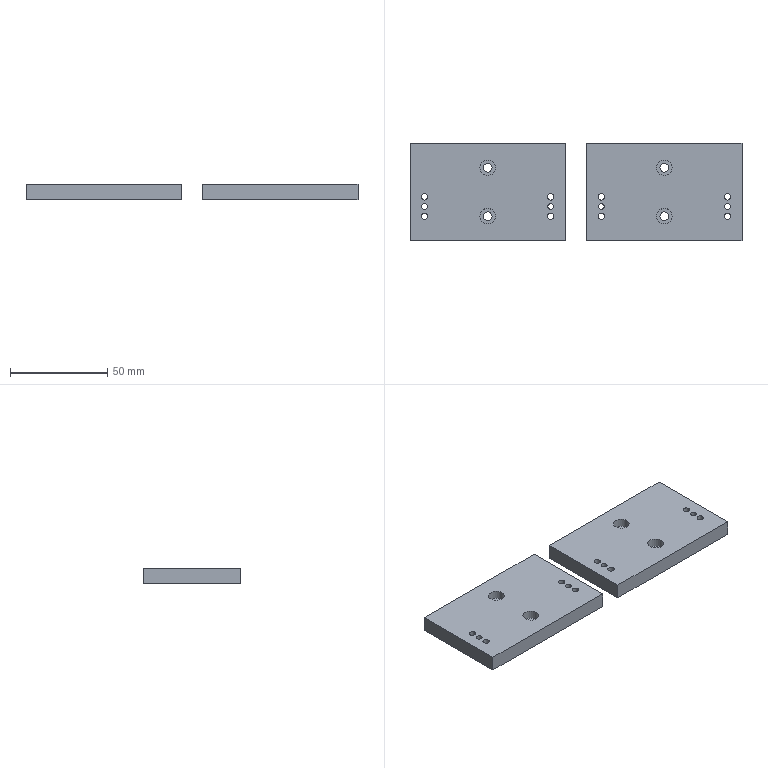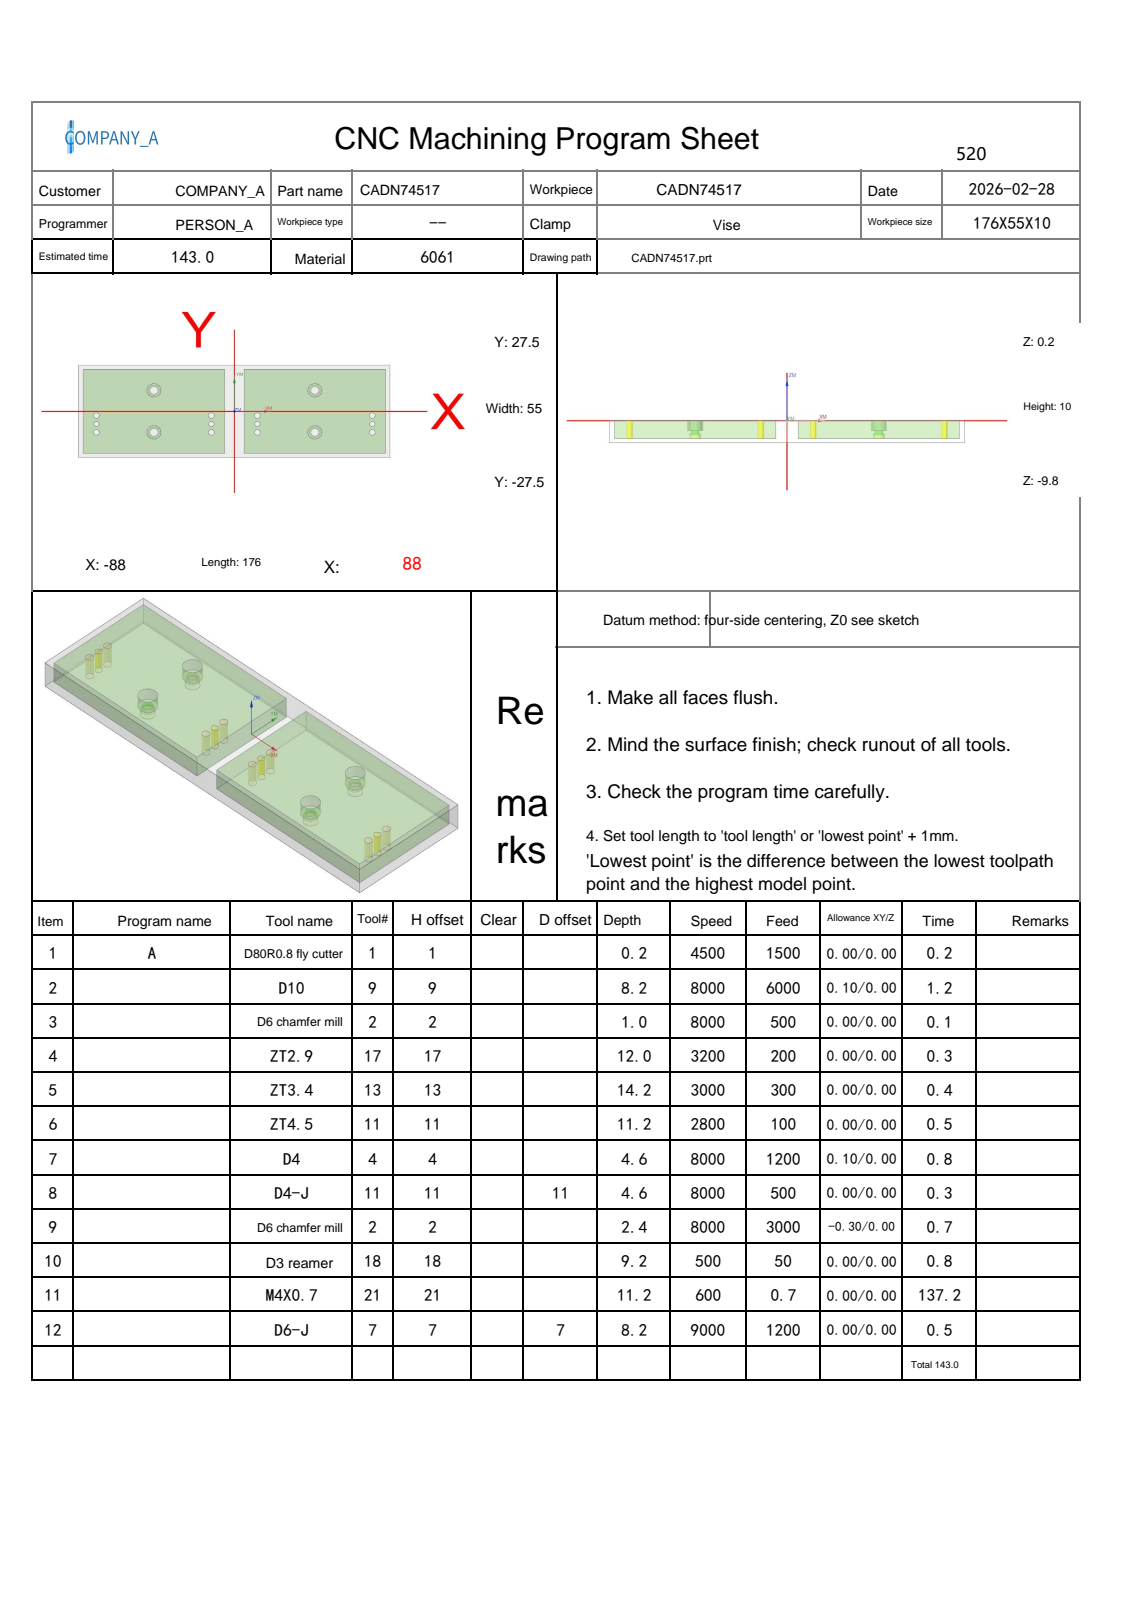NC program | NX | posted by the shop | part box 171 x 50 x 8 mm
Whole program:
%
O0001
(Machine time: 271.00 MIN)
(===Total Tool:10===)
(T1=D80R0.8 fly cutter D=80.  R=0.8  D-  H01 Z=0.    )
(T9=D10     D=10.  R=0.   D-  H09 Z=-8.   )
(T2=D6 chamfer mill   D=6.   R=0.   D-  H02 Z=-2.2  )
(T17=ZT2.9  D=2.9  DR_a=120 D-  H17 Z=-11.84)
(T13=ZT3.4  D=3.4  DR_a=118 D-  H13 Z=-14.  )
(T11=ZT4.5  D=4.5  DR_a=118 D-  H11 Z=-11.  )
(T4=D4      D=4.   R=0.   D-  H04 Z=-4.4  )
(T18=D3 reamer   D=3.   DR_a=180 D-  H18 Z=-9.   )
(T21=M4X0.7 D=3.3  DR_a=180 D-  H21 Z=-11.  )
(T7=D6-J    D=6.   R=0.   D7  H07 Z=-8.   )
G80 G90 G17 G49 G40
G91 G28 Z0
M01
N1 T01 M06
(D80R0.8 fly cutter  D=80. R=0.8 H=01 ce=0.00 di=0.00)
G00 G90 G54 X-130.5 Y0.0 M03 S4500
G43 H01 Z50.
M08
Z2.
G01 Z0.0 F1500.
X-125.5
X125.5
X130.5
Z2.
G00 Z50.
G91 G28 Z0.0
M05
M09
G91 G28 Z0.0
M01
N2 T09 M06
(D10  D=10. R=0. H=09 ce=0.10 di=0.00)
G00 G90 G54 X-45.5 Y-30.1 M03 S8000
G43 H09 Z50.
M08
Z.5
G01 X-85.5 Z.394 F6000.
G02 X-90.6 Y-25. Z.373 I0.0 J5.1
G01 Y25. Z.241
G02 X-85.5 Y30.1 Z.219 I5.1 J0.0
G01 X-5.5 Z.008
G02 X-.4 Y25. Z-.013 I0.0 J-5.1
G01 Y-25. Z-.146
G02 X-5.5 Y-30.1 Z-.167 I-5.1 J0.0
G01 X-85.5 Z-.379
G02 X-90.6 Y-25. Z-.4 I0.0 J5.1
G01 Y25. Z-.532
G02 X-85.5 Y30.1 Z-.553 I5.1 J0.0
G01 X-5.5 Z-.765
G02 X-.4 Y25. Z-.786 I0.0 J-5.1
G01 Y-25. Z-.918
G02 X-5.5 Y-30.1 Z-.94 I-5.1 J0.0
G01 X-85.5 Z-1.151
G02 X-90.6 Y-25. Z-1.172 I0.0 J5.1
G01 Y25. Z-1.305
G02 X-85.5 Y30.1 Z-1.326 I5.1 J0.0
G01 X-5.5 Z-1.538
G02 X-.4 Y25. Z-1.559 I0.0 J-5.1
G01 Y-25. Z-1.691
G02 X-5.5 Y-30.1 Z-1.712 I-5.1 J0.0
G01 X-85.5 Z-1.924
G02 X-90.6 Y-25. Z-1.945 I0.0 J5.1
G01 Y25. Z-2.078
G02 X-85.5 Y30.1 Z-2.099 I5.1 J0.0
G01 X-5.5 Z-2.31
G02 X-.4 Y25. Z-2.332 I0.0 J-5.1
G01 Y-25. Z-2.464
G02 X-5.5 Y-30.1 Z-2.485 I-5.1 J0.0
G01 X-85.5 Z-2.697
G02 X-90.6 Y-25. Z-2.718 I0.0 J5.1
G01 Y25. Z-2.85
G02 X-85.5 Y30.1 Z-2.871 I5.1 J0.0
G01 X-5.5 Z-3.083
G02 X-.4 Y25. Z-3.104 I0.0 J-5.1
G01 Y-25. Z-3.237
G02 X-5.5 Y-30.1 Z-3.258 I-5.1 J0.0
G01 X-85.5 Z-3.469
G02 X-90.6 Y-25. Z-3.491 I0.0 J5.1
G01 Y25. Z-3.623
G02 X-85.5 Y30.1 Z-3.644 I5.1 J0.0
G01 X-5.5 Z-3.856
G02 X-.4 Y25. Z-3.877 I0.0 J-5.1
G01 Y-25. Z-4.009
G02 X-5.5 Y-30.1 Z-4.031 I-5.1 J0.0
G01 X-85.5 Z-4.242
G02 X-90.6 Y-25. Z-4.263 I0.0 J5.1
G01 Y25. Z-4.396
G02 X-85.5 Y30.1 Z-4.417 I5.1 J0.0
G01 X-5.5 Z-4.629
G02 X-.4 Y25. Z-4.65 I0.0 J-5.1
G01 Y-25. Z-4.782
G02 X-5.5 Y-30.1 Z-4.803 I-5.1 J0.0
G01 X-85.5 Z-5.015
G02 X-90.6 Y-25. Z-5.036 I0.0 J5.1
G01 Y25. Z-5.168
G02 X-85.5 Y30.1 Z-5.19 I5.1 J0.0
G01 X-5.5 Z-5.401
G02 X-.4 Y25. Z-5.422 I0.0 J-5.1
G01 Y-25. Z-5.555
G02 X-5.5 Y-30.1 Z-5.576 I-5.1 J0.0
G01 X-85.5 Z-5.788
G02 X-90.6 Y-25. Z-5.809 I0.0 J5.1
G01 Y25. Z-5.941
G02 X-85.5 Y30.1 Z-5.962 I5.1 J0.0
G01 X-5.5 Z-6.174
G02 X-.4 Y25. Z-6.195 I0.0 J-5.1
G01 Y-25. Z-6.328
G02 X-5.5 Y-30.1 Z-6.349 I-5.1 J0.0
G01 X-85.5 Z-6.56
G02 X-90.6 Y-25. Z-6.582 I0.0 J5.1
G01 Y25. Z-6.714
G02 X-85.5 Y30.1 Z-6.735 I5.1 J0.0
G01 X-5.5 Z-6.947
G02 X-.4 Y25. Z-6.968 I0.0 J-5.1
G01 Y-25. Z-7.1
G02 X-5.5 Y-30.1 Z-7.121 I-5.1 J0.0
G01 X-85.5 Z-7.333
G02 X-90.6 Y-25. Z-7.354 I0.0 J5.1
G01 Y25. Z-7.487
G02 X-85.5 Y30.1 Z-7.508 I5.1 J0.0
G01 X-5.5 Z-7.719
G02 X-.4 Y25. Z-7.741 I0.0 J-5.1
G01 Y-25. Z-7.873
G02 X-5.5 Y-30.1 Z-7.894 I-5.1 J0.0
G01 X-45.5 Z-8.
X-85.5
G02 X-90.6 Y-25. I0.0 J5.1
G01 Y25.
G02 X-85.5 Y30.1 I5.1 J0.0
G01 X-5.5
G02 X-.4 Y25. I0.0 J-5.1
G01 Y-25.
G02 X-5.5 Y-30.1 I-5.1 J0.0
G01 X-45.5
X-46.
Z-7.
G00 Z50.
X45.5
Z.5
G01 X5.5 Z.394
G02 X.4 Y-25. Z.373 I0.0 J5.1
G01 Y25. Z.241
G02 X5.5 Y30.1 Z.219 I5.1 J0.0
G01 X85.5 Z.008
G02 X90.6 Y25. Z-.013 I0.0 J-5.1
G01 Y-25. Z-.146
G02 X85.5 Y-30.1 Z-.167 I-5.1 J0.0
G01 X5.5 Z-.379
G02 X.4 Y-25. Z-.4 I0.0 J5.1
G01 Y25. Z-.532
G02 X5.5 Y30.1 Z-.553 I5.1 J0.0
G01 X85.5 Z-.765
G02 X90.6 Y25. Z-.786 I0.0 J-5.1
G01 Y-25. Z-.918
G02 X85.5 Y-30.1 Z-.94 I-5.1 J0.0
G01 X5.5 Z-1.151
G02 X.4 Y-25. Z-1.172 I0.0 J5.1
G01 Y25. Z-1.305
G02 X5.5 Y30.1 Z-1.326 I5.1 J0.0
G01 X85.5 Z-1.538
G02 X90.6 Y25. Z-1.559 I0.0 J-5.1
G01 Y-25. Z-1.691
G02 X85.5 Y-30.1 Z-1.712 I-5.1 J0.0
G01 X5.5 Z-1.924
G02 X.4 Y-25. Z-1.945 I0.0 J5.1
G01 Y25. Z-2.078
G02 X5.5 Y30.1 Z-2.099 I5.1 J0.0
G01 X85.5 Z-2.31
G02 X90.6 Y25. Z-2.332 I0.0 J-5.1
G01 Y-25. Z-2.464
G02 X85.5 Y-30.1 Z-2.485 I-5.1 J0.0
G01 X5.5 Z-2.697
G02 X.4 Y-25. Z-2.718 I0.0 J5.1
G01 Y25. Z-2.85
G02 X5.5 Y30.1 Z-2.871 I5.1 J0.0
G01 X85.5 Z-3.083
G02 X90.6 Y25. Z-3.104 I0.0 J-5.1
G01 Y-25. Z-3.237
G02 X85.5 Y-30.1 Z-3.258 I-5.1 J0.0
G01 X5.5 Z-3.469
G02 X.4 Y-25. Z-3.491 I0.0 J5.1
G01 Y25. Z-3.623
G02 X5.5 Y30.1 Z-3.644 I5.1 J0.0
G01 X85.5 Z-3.856
G02 X90.6 Y25. Z-3.877 I0.0 J-5.1
G01 Y-25. Z-4.009
G02 X85.5 Y-30.1 Z-4.031 I-5.1 J0.0
G01 X5.5 Z-4.242
G02 X.4 Y-25. Z-4.263 I0.0 J5.1
G01 Y25. Z-4.396
G02 X5.5 Y30.1 Z-4.417 I5.1 J0.0
G01 X85.5 Z-4.629
G02 X90.6 Y25. Z-4.65 I0.0 J-5.1
G01 Y-25. Z-4.782
G02 X85.5 Y-30.1 Z-4.803 I-5.1 J0.0
G01 X5.5 Z-5.015
G02 X.4 Y-25. Z-5.036 I0.0 J5.1
G01 Y25. Z-5.168
G02 X5.5 Y30.1 Z-5.19 I5.1 J0.0
G01 X85.5 Z-5.401
G02 X90.6 Y25. Z-5.422 I0.0 J-5.1
G01 Y-25. Z-5.555
G02 X85.5 Y-30.1 Z-5.576 I-5.1 J0.0
G01 X5.5 Z-5.788
G02 X.4 Y-25. Z-5.809 I0.0 J5.1
G01 Y25. Z-5.941
G02 X5.5 Y30.1 Z-5.962 I5.1 J0.0
G01 X85.5 Z-6.174
G02 X90.6 Y25. Z-6.195 I0.0 J-5.1
G01 Y-25. Z-6.328
G02 X85.5 Y-30.1 Z-6.349 I-5.1 J0.0
G01 X5.5 Z-6.56
G02 X.4 Y-25. Z-6.582 I0.0 J5.1
G01 Y25. Z-6.714
G02 X5.5 Y30.1 Z-6.735 I5.1 J0.0
G01 X85.5 Z-6.947
G02 X90.6 Y25. Z-6.968 I0.0 J-5.1
G01 Y-25. Z-7.1
G02 X85.5 Y-30.1 Z-7.121 I-5.1 J0.0
G01 X5.5 Z-7.333
G02 X.4 Y-25. Z-7.354 I0.0 J5.1
G01 Y25. Z-7.487
G02 X5.5 Y30.1 Z-7.508 I5.1 J0.0
G01 X85.5 Z-7.719
G02 X90.6 Y25. Z-7.741 I0.0 J-5.1
G01 Y-25. Z-7.873
G02 X85.5 Y-30.1 Z-7.894 I-5.1 J0.0
G01 X45.5 Z-8.
X5.5
G02 X.4 Y-25. I0.0 J5.1
G01 Y25.
G02 X5.5 Y30.1 I5.1 J0.0
G01 X85.5
G02 X90.6 Y25. I0.0 J-5.1
G01 Y-25.
G02 X85.5 Y-30.1 I-5.1 J0.0
G01 X45.5
X45.
Z-7.
G00 Z50.
G91 G28 Z0.0
M05
M09
G91 G28 Z0.0
M01
N3 T02 M06
(D6 chamfer mill  D=6. R=0. H=02 ce=0.00 di=0.00)
G00 G90 G54 X-78. Y-2.5 M03 S8000
G43 H02 Z50.
M08
G98 G81 X-78. Y-2.5 Z-.8 R1. F500.
Y-7.5
Y-12.5
X-45.5
Y12.5
X-13. Y-2.5
Y-7.5
Y-12.5
X13.
Y-7.5
Y-2.5
X45.5 Y12.5
Y-12.5
X78.
Y-7.5
Y-2.5
G80
G00 Z50.
G91 G28 Z0.0
M05
M09
G91 G28 Z0.0
M01
N4 T17 M06
(ZT2.9 D=2.9 DR_a=120 H=17)
G00 G90 G54 X78. Y-7.5 M03 S3200
G43 H17 Z50.
M08
G98 G83 X78. Y-7.5 Z-11.837 R1. F200. Q2.
X13.
X-13.
X-78.
G80
G00 Z50.
G91 G28 Z0.0
M05
M09
G91 G28 Z0.0
M01
N5 T13 M06
(ZT3.4 D=3.4 DR_a=118 H=13)
G00 G90 G54 X-78. Y-12.5 M03 S3000
G43 H13 Z50.
M08
G98 G83 X-78. Y-12.5 Z-14. R1. F300. Q2.
Y-2.5
X-13.
Y-12.5
X13.
Y-2.5
X78.
Y-12.5
G80
G00 Z50.
G91 G28 Z0.0
M05
M09
G91 G28 Z0.0
M01
N6 T11 M06
(ZT4.5 D=4.5 DR_a=118 H=11)
G00 G90 G54 X45.5 Y-12.5 M03 S2800
G43 H11 Z50.
M08
G98 G83 X45.5 Y-12.5 Z-11. R1. F100. Q2.
Y12.5
X-45.5
Y-12.5
G80
G00 Z50.
G91 G28 Z0.0
M05
M09
G91 G28 Z0.0
M01
N7 T04 M06
(D4  D=4. R=0. H=04 ce=0.10 di=0.00)
G00 G90 G54 X45.5 Y-12.5 M03 S8000
G43 H04 Z50.
M08
Z.5
G03 X46.45 Y-13.45 I.95 J0.0 F1200.
X47.4 Y-12.5 I0.0 J.95
X47.4 Y-12.5 Z.2 I-1.9 J0.0
X47.4 Y-12.5 Z-.1 I-1.9 J0.0
X47.4 Y-12.5 Z-.4 I-1.9 J0.0
X47.4 Y-12.5 Z-.7 I-1.9 J0.0
X47.4 Y-12.5 Z-1. I-1.9 J0.0
X47.4 Y-12.5 Z-1.3 I-1.9 J0.0
X47.4 Y-12.5 Z-1.6 I-1.9 J0.0
X47.4 Y-12.5 Z-1.9 I-1.9 J0.0
X47.4 Y-12.5 Z-2.2 I-1.9 J0.0
X47.4 Y-12.5 Z-2.5 I-1.9 J0.0
X47.4 Y-12.5 Z-2.8 I-1.9 J0.0
X47.4 Y-12.5 Z-3.1 I-1.9 J0.0
X47.4 Y-12.5 Z-3.4 I-1.9 J0.0
X47.4 Y-12.5 Z-3.7 I-1.9 J0.0
X47.4 Y-12.5 Z-4. I-1.9 J0.0
X47.4 Y-12.5 Z-4.3 I-1.9 J0.0
X44.55 Y-10.855 Z-4.4 I-1.9 J0.0
X43.6 Y-12.5 I.95 J-1.645
X45.5 Y-14.4 I1.9 J0.0
X47.4 Y-12.5 I0.0 J1.9
X45.5 Y-10.6 I-1.9 J0.0
X44.55 Y-10.855 I0.0 J-1.9
X44.075 Y-11.677 I.475 J-.823
X45.025 Y-12.627 I.95 J0.0
X45.5 Y-12.5 I0.0 J.95
G00 Z50.
Y12.5
Z.5
G03 X46.45 Y11.55 I.95 J0.0
X47.4 Y12.5 I0.0 J.95
X47.4 Y12.5 Z.2 I-1.9 J0.0
X47.4 Y12.5 Z-.1 I-1.9 J0.0
X47.4 Y12.5 Z-.4 I-1.9 J0.0
X47.4 Y12.5 Z-.7 I-1.9 J0.0
X47.4 Y12.5 Z-1. I-1.9 J0.0
X47.4 Y12.5 Z-1.3 I-1.9 J0.0
X47.4 Y12.5 Z-1.6 I-1.9 J0.0
X47.4 Y12.5 Z-1.9 I-1.9 J0.0
X47.4 Y12.5 Z-2.2 I-1.9 J0.0
X47.4 Y12.5 Z-2.5 I-1.9 J0.0
X47.4 Y12.5 Z-2.8 I-1.9 J0.0
X47.4 Y12.5 Z-3.1 I-1.9 J0.0
X47.4 Y12.5 Z-3.4 I-1.9 J0.0
X47.4 Y12.5 Z-3.7 I-1.9 J0.0
X47.4 Y12.5 Z-4. I-1.9 J0.0
X47.4 Y12.5 Z-4.3 I-1.9 J0.0
X44.55 Y14.145 Z-4.4 I-1.9 J0.0
X43.6 Y12.5 I.95 J-1.645
X45.5 Y10.6 I1.9 J0.0
X47.4 Y12.5 I0.0 J1.9
X45.5 Y14.4 I-1.9 J0.0
X44.55 Y14.145 I0.0 J-1.9
X44.075 Y13.323 I.475 J-.823
X45.025 Y12.373 I.95 J0.0
X45.5 Y12.5 I0.0 J.95
G00 Z50.
X-45.5
Z.5
G03 X-44.55 Y11.55 I.95 J0.0
X-43.6 Y12.5 I0.0 J.95
X-43.6 Y12.5 Z.2 I-1.9 J0.0
X-43.6 Y12.5 Z-.1 I-1.9 J0.0
X-43.6 Y12.5 Z-.4 I-1.9 J0.0
X-43.6 Y12.5 Z-.7 I-1.9 J0.0
X-43.6 Y12.5 Z-1. I-1.9 J0.0
X-43.6 Y12.5 Z-1.3 I-1.9 J0.0
X-43.6 Y12.5 Z-1.6 I-1.9 J0.0
X-43.6 Y12.5 Z-1.9 I-1.9 J0.0
X-43.6 Y12.5 Z-2.2 I-1.9 J0.0
X-43.6 Y12.5 Z-2.5 I-1.9 J0.0
X-43.6 Y12.5 Z-2.8 I-1.9 J0.0
X-43.6 Y12.5 Z-3.1 I-1.9 J0.0
X-43.6 Y12.5 Z-3.4 I-1.9 J0.0
X-43.6 Y12.5 Z-3.7 I-1.9 J0.0
X-43.6 Y12.5 Z-4. I-1.9 J0.0
X-43.6 Y12.5 Z-4.3 I-1.9 J0.0
X-46.45 Y14.145 Z-4.4 I-1.9 J0.0
X-47.4 Y12.5 I.95 J-1.645
X-45.5 Y10.6 I1.9 J0.0
X-43.6 Y12.5 I0.0 J1.9
X-45.5 Y14.4 I-1.9 J0.0
X-46.45 Y14.145 I0.0 J-1.9
X-46.925 Y13.323 I.475 J-.823
X-45.975 Y12.373 I.95 J0.0
X-45.5 Y12.5 I0.0 J.95
G00 Z50.
Y-12.5
Z.5
G03 X-44.55 Y-13.45 I.95 J0.0
X-43.6 Y-12.5 I0.0 J.95
X-43.6 Y-12.5 Z.2 I-1.9 J0.0
X-43.6 Y-12.5 Z-.1 I-1.9 J0.0
X-43.6 Y-12.5 Z-.4 I-1.9 J0.0
X-43.6 Y-12.5 Z-.7 I-1.9 J0.0
X-43.6 Y-12.5 Z-1. I-1.9 J0.0
X-43.6 Y-12.5 Z-1.3 I-1.9 J0.0
X-43.6 Y-12.5 Z-1.6 I-1.9 J0.0
X-43.6 Y-12.5 Z-1.9 I-1.9 J0.0
X-43.6 Y-12.5 Z-2.2 I-1.9 J0.0
X-43.6 Y-12.5 Z-2.5 I-1.9 J0.0
X-43.6 Y-12.5 Z-2.8 I-1.9 J0.0
X-43.6 Y-12.5 Z-3.1 I-1.9 J0.0
X-43.6 Y-12.5 Z-3.4 I-1.9 J0.0
X-43.6 Y-12.5 Z-3.7 I-1.9 J0.0
X-43.6 Y-12.5 Z-4. I-1.9 J0.0
X-43.6 Y-12.5 Z-4.3 I-1.9 J0.0
X-46.45 Y-10.855 Z-4.4 I-1.9 J0.0
X-47.4 Y-12.5 I.95 J-1.645
X-45.5 Y-14.4 I1.9 J0.0
X-43.6 Y-12.5 I0.0 J1.9
X-45.5 Y-10.6 I-1.9 J0.0
X-46.45 Y-10.855 I0.0 J-1.9
X-46.925 Y-11.677 I.475 J-.823
X-45.975 Y-12.627 I.95 J0.0
X-45.5 Y-12.5 I0.0 J.95
G00 Z50.
G91 G28 Z0.0
M05
M09
G91 G28 Z0.0
M01
N8 T11 M06
(D4-J  D=4. R=0. H=11 ce=0.00 di=0.00)
G00 G90 G54 X45.5 Y-12.5 M03 S8000
G43 H11 Z50.
M08
Z.5
G41 D11
G01 X45.54 Y-12.696 F500.
G03 X46.51 Y-13.49 I.97 J.196
X47.5 Y-12.5 I0.0 J.99
X47.484 Y-12.751 Z-4.4 I-2. J0.0
X47.5 Y-12.5 I-1.984 J.251
X45.5 Y-10.5 I-2. J0.0
X43.5 Y-12.5 I0.0 J-2.
X45.5 Y-14.5 I2. J0.0
X47.484 Y-12.751 I0.0 J2.
G01 X47.492 Y-12.627
G03 X46.502 Y-11.637 I-.99 J0.0
X45.564 Y-12.31 I0.0 J-.99
G01 G40 X45.5 Y-12.5
G00 Z50.
Y12.5
Z.5
G41 D11
G01 X45.54 Y12.304
G03 X46.51 Y11.51 I.97 J.196
X47.5 Y12.5 I0.0 J.99
X47.484 Y12.249 Z-4.4 I-2. J0.0
X47.5 Y12.5 I-1.984 J.251
X45.5 Y14.5 I-2. J0.0
X43.5 Y12.5 I0.0 J-2.
X45.5 Y10.5 I2. J0.0
X47.484 Y12.249 I0.0 J2.
G01 X47.492 Y12.373
G03 X46.502 Y13.363 I-.99 J0.0
X45.564 Y12.69 I0.0 J-.99
G01 G40 X45.5 Y12.5
G00 Z50.
X-45.5
Z.5
G41 D11
G01 X-45.46 Y12.304
G03 X-44.49 Y11.51 I.97 J.196
X-43.5 Y12.5 I0.0 J.99
X-43.516 Y12.249 Z-4.4 I-2. J0.0
X-43.5 Y12.5 I-1.984 J.251
X-45.5 Y14.5 I-2. J0.0
X-47.5 Y12.5 I0.0 J-2.
X-45.5 Y10.5 I2. J0.0
X-43.516 Y12.249 I0.0 J2.
G01 X-43.508 Y12.373
G03 X-44.498 Y13.363 I-.99 J0.0
X-45.436 Y12.69 I0.0 J-.99
G01 G40 X-45.5 Y12.5
G00 Z50.
Y-12.5
Z.5
G41 D11
G01 X-45.46 Y-12.696
G03 X-44.49 Y-13.49 I.97 J.196
X-43.5 Y-12.5 I0.0 J.99
X-43.516 Y-12.751 Z-4.4 I-2. J0.0
X-43.5 Y-12.5 I-1.984 J.251
X-45.5 Y-10.5 I-2. J0.0
X-47.5 Y-12.5 I0.0 J-2.
X-45.5 Y-14.5 I2. J0.0
X-43.516 Y-12.751 I0.0 J2.
G01 X-43.508 Y-12.627
G03 X-44.498 Y-11.637 I-.99 J0.0
X-45.436 Y-12.31 I0.0 J-.99
G01 G40 X-45.5 Y-12.5
G00 Z50.
G91 G28 Z0.0
M05
M09
G91 G28 Z0.0
M01
N9 T02 M06
(D6 chamfer mill  D=6. R=0. H=02 ce=0.00 di=0.00)
G00 G90 G54 X-45.25 Y-27.128 M03 S8000
G43 H02 Z50.
M08
Z2.099
G01 Z-1.5 F3000.
G03 X-45.17 Y-26.828 I-.52 J.3
X-45.47 Y-26.308 I-.6 J0.0
G01 X-45.5 Y-26.3
X-85.5
G02 X-86.8 Y-25. I0.0 J1.3
G01 Y25.
G02 X-85.5 Y26.3 I1.3 J0.0
G01 X-5.5
G02 X-4.2 Y25. I0.0 J-1.3
G01 Y-25.
G02 X-5.5 Y-26.3 I-1.3 J0.0
G01 X-45.5
X-45.53 Y-26.308
G03 X-45.83 Y-26.828 I.3 J-.52
X-45.75 Y-27.128 I.6 J0.0
G01 Z2.099
G00 Z50.
X45.75
Z2.099
G01 Z-1.5
G03 X45.83 Y-26.828 I-.52 J.3
X45.53 Y-26.308 I-.6 J0.0
G01 X45.5 Y-26.3
X5.5
G02 X4.2 Y-25. I0.0 J1.3
G01 Y25.
G02 X5.5 Y26.3 I1.3 J0.0
G01 X85.5
G02 X86.8 Y25. I0.0 J-1.3
G01 Y-25.
G02 X85.5 Y-26.3 I-1.3 J0.0
G01 X45.5
X45.47 Y-26.308
G03 X45.17 Y-26.828 I.3 J-.52
X45.25 Y-27.128 I.6 J0.0
G01 Z2.099
G00 Z50.
G00 G90 X78. Y-7.5 M03 S8000
Z50.
G98 G81 X78. Y-7.5 Z-1.8 R3. F500.
X13.
X-13.
X-78.
G80
G00 Z50.
G00 G90 X-78. Y-12.5 M03 S8000
Z50.
G98 G81 X-78. Y-12.5 Z-2.2 R3. F500.
Y-2.5
X-13.
Y-12.5
X13.
Y-2.5
X78.
Y-12.5
G80
G00 Z50.
G00 G90 X-48.712 Y-13.247 M03 S8000
Z50.
Z2.5
G01 X-48.66 Y-13.462 Z2.42 F500.
X-48.524 Y-13.828 Z2.278
X-48.347 Y-14.175 Z2.136
X-48.129 Y-14.499 Z1.994
X-47.875 Y-14.795 Z1.852
X-47.588 Y-15.059 Z1.71
X-47.272 Y-15.288 Z1.568
X-47.028 Y-15.428 Z1.465
X-46.672 Y-15.588 Z1.323
X-46.3 Y-15.705 Z1.181
X-45.916 Y-15.777 Z1.039
X-45.527 Y-15.803 Z.897
X-45.138 Y-15.783 Z.755
X-44.753 Y-15.717 Z.613
X-44.379 Y-15.607 Z.471
X-44.02 Y-15.453 Z.329
X-43.682 Y-15.258 Z.187
X-43.37 Y-15.024 Z.045
X-43.087 Y-14.756 Z-.097
X-42.838 Y-14.455 Z-.239
X-42.626 Y-14.128 Z-.381
X-42.454 Y-13.778 Z-.523
X-42.325 Y-13.41 Z-.665
X-42.24 Y-13.029 Z-.807
X-42.2 Y-12.641 Z-.949
Y-12.5 Z-1.
G03 X-45.5 Y-9.2 I-3.3 J0.0
X-48.8 Y-12.5 I0.0 J-3.3
X-45.5 Y-15.8 I3.3 J0.0
X-42.2 Y-12.5 I0.0 J3.3
X-42.238 Y-12.002 I-3.3 J0.0
G01 Z1.5
G00 Z50.
X-48.712 Y11.753
Z2.5
G01 X-48.66 Y11.538 Z2.42
X-48.524 Y11.172 Z2.278
X-48.347 Y10.825 Z2.136
X-48.129 Y10.501 Z1.994
X-47.875 Y10.205 Z1.852
X-47.588 Y9.941 Z1.71
X-47.272 Y9.712 Z1.568
X-47.028 Y9.572 Z1.465
X-46.672 Y9.412 Z1.323
X-46.3 Y9.295 Z1.181
X-45.916 Y9.223 Z1.039
X-45.527 Y9.197 Z.897
X-45.138 Y9.217 Z.755
X-44.753 Y9.283 Z.613
X-44.379 Y9.393 Z.471
X-44.02 Y9.547 Z.329
X-43.682 Y9.742 Z.187
X-43.37 Y9.976 Z.045
X-43.087 Y10.244 Z-.097
X-42.838 Y10.545 Z-.239
X-42.626 Y10.872 Z-.381
X-42.454 Y11.222 Z-.523
X-42.325 Y11.59 Z-.665
X-42.24 Y11.971 Z-.807
X-42.2 Y12.359 Z-.949
Y12.5 Z-1.
G03 X-45.5 Y15.8 I-3.3 J0.0
X-48.8 Y12.5 I0.0 J-3.3
X-45.5 Y9.2 I3.3 J0.0
X-42.2 Y12.5 I0.0 J3.3
X-42.238 Y12.998 I-3.3 J0.0
G01 Z1.5
G00 Z50.
X42.288 Y11.753
Z2.5
G01 X42.34 Y11.538 Z2.42
X42.476 Y11.172 Z2.278
X42.653 Y10.825 Z2.136
X42.871 Y10.501 Z1.994
X43.125 Y10.205 Z1.852
X43.412 Y9.941 Z1.71
X43.728 Y9.712 Z1.568
X43.972 Y9.572 Z1.465
X44.328 Y9.412 Z1.323
X44.7 Y9.295 Z1.181
X45.084 Y9.223 Z1.039
X45.473 Y9.197 Z.897
X45.862 Y9.217 Z.755
X46.247 Y9.283 Z.613
X46.621 Y9.393 Z.471
X46.98 Y9.547 Z.329
X47.318 Y9.742 Z.187
X47.63 Y9.976 Z.045
X47.913 Y10.244 Z-.097
X48.162 Y10.545 Z-.239
X48.374 Y10.872 Z-.381
X48.546 Y11.222 Z-.523
X48.675 Y11.59 Z-.665
X48.76 Y11.971 Z-.807
X48.8 Y12.359 Z-.949
Y12.5 Z-1.
G03 X45.5 Y15.8 I-3.3 J0.0
X42.2 Y12.5 I0.0 J-3.3
X45.5 Y9.2 I3.3 J0.0
X48.8 Y12.5 I0.0 J3.3
X48.762 Y12.998 I-3.3 J0.0
G01 Z1.5
G00 Z50.
X42.288 Y-13.247
Z2.5
G01 X42.34 Y-13.462 Z2.42
X42.476 Y-13.828 Z2.278
X42.653 Y-14.175 Z2.136
X42.871 Y-14.499 Z1.994
X43.125 Y-14.795 Z1.852
X43.412 Y-15.059 Z1.71
X43.728 Y-15.288 Z1.568
X43.972 Y-15.428 Z1.465
X44.328 Y-15.588 Z1.323
X44.7 Y-15.705 Z1.181
X45.084 Y-15.777 Z1.039
X45.473 Y-15.803 Z.897
X45.862 Y-15.783 Z.755
X46.247 Y-15.717 Z.613
X46.621 Y-15.607 Z.471
X46.98 Y-15.453 Z.329
X47.318 Y-15.258 Z.187
X47.63 Y-15.024 Z.045
X47.913 Y-14.756 Z-.097
X48.162 Y-14.455 Z-.239
X48.374 Y-14.128 Z-.381
X48.546 Y-13.778 Z-.523
X48.675 Y-13.41 Z-.665
X48.76 Y-13.029 Z-.807
X48.8 Y-12.641 Z-.949
Y-12.5 Z-1.
G03 X45.5 Y-9.2 I-3.3 J0.0
X42.2 Y-12.5 I0.0 J-3.3
X45.5 Y-15.8 I3.3 J0.0
X48.8 Y-12.5 I0.0 J3.3
X48.762 Y-12.002 I-3.3 J0.0
G01 Z1.5
G00 Z50.
G91 G28 Z0.0
M05
M09
G91 G28 Z0.0
M01
N10 T18 M06
(D3 reamer D=3. DR_a=180 H=18)
G00 G90 G54 X78. Y-7.5 M03 S500
G43 H18 Z50.
M08
G98 G81 X78. Y-7.5 Z-9. R1. F50.
X13.
X-13.
X-78.
G80
G00 Z50.
G91 G28 Z0.0
M05
M09
G91 G28 Z0.0
M01
N11 T21 M06
(M4X0.7 D=3.3 DR_a=180 H=21)
G00 G90 G54 X-78. Y-12.5 M03 S600
G43 H21 Z50.
M08
G95
G98 G84 X-78. Y-12.5 Z-11. R1. F.7 Q4.
Y-2.5
X-13.
Y-12.5
X13.
Y-2.5
X78.
Y-12.5
G80
G94
G00 Z50.
G91 G28 Z0.0
M05
M09
G91 G28 Z0.0
M01
N12 T07 M06
(D6-J  D=6. R=0. H=07 ce=0.00 di=0.00)
G00 G90 G54 X-4.483 Y-29.073 M03 S9000
G43 H07 Z50.
M08
Z-7.5
G01 Z-8. F1200.
G41 D07
X-4.508 Y-28.875
G03 X-5.5 Y-28. I-.992 J-.125
G01 X-85.5
G02 X-88.5 Y-25. I0.0 J3.
G01 Y25.
G02 X-85.5 Y28. I3. J0.0
G01 X-5.5
G02 X-2.5 Y25. I0.0 J-3.
G01 Y-25.
G02 X-5.5 Y-28. I-3. J0.0
G01 X-6.
G03 X-7. Y-29. I0.0 J-1.
G01 G40 Y-29.2
Z-7.5
G00 Z50.
X86.517 Y-29.073
Z-7.5
G01 Z-8.
G41 D07
X86.492 Y-28.875
G03 X85.5 Y-28. I-.992 J-.125
G01 X5.5
G02 X2.5 Y-25. I0.0 J3.
G01 Y25.
G02 X5.5 Y28. I3. J0.0
G01 X85.5
G02 X88.5 Y25. I0.0 J-3.
G01 Y-25.
G02 X85.5 Y-28. I-3. J0.0
G01 X85.
G03 X84. Y-29. I0.0 J-1.
G01 G40 Y-29.2
Z-7.5
G00 Z50.
M05
M09
G91 G28 Z0.0
G91 G28 Y0.0
M30
%